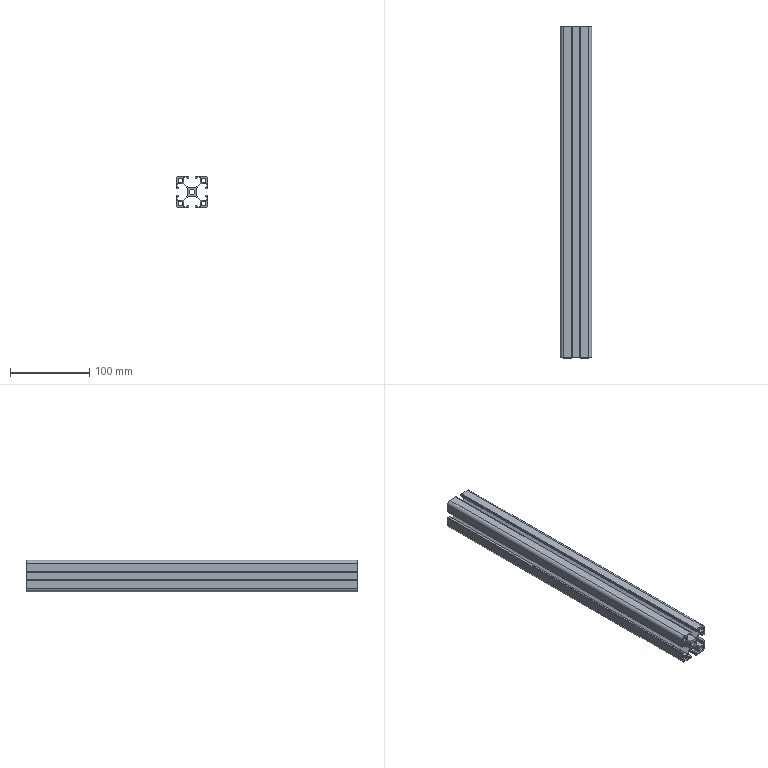Part | SolidWorks | features BaseBody 1 | 1 solid | 104 faces | box 40 x 420 x 40 mm | volume 199444 mm3 | plane 94 | cylinder 10 | commonest cylinder face diameters 5 x4 9 x4 6.8 x2